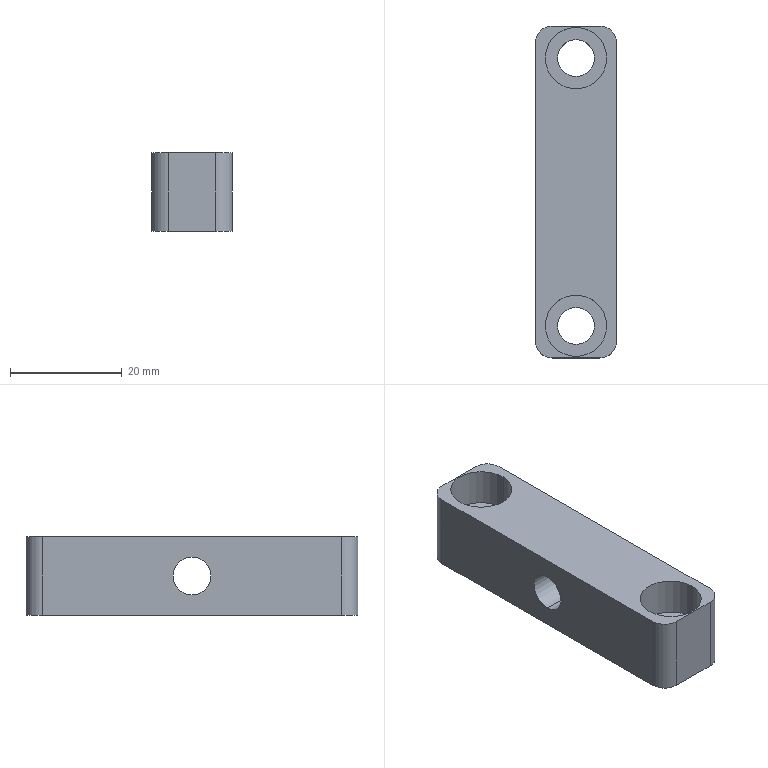Part | SolidWorks | features HoleWzd 2, Extrusion 1, Fillet 1 | 1 solid | 22 faces | box 14.5 x 59.5 x 14 mm | volume 9659 mm3 | cylinder 14 | plane 8 | commonest cylinder face diameters 6 x4 6.6 x4 11 x4 6.8 x2
STEP:
#1=CARTESIAN_POINT('',(7.25,0.,3.6));
#2=VERTEX_POINT('',#1);
#3=CARTESIAN_POINT('',(7.25,0.,10.4));
#4=VERTEX_POINT('',#3);
#5=CARTESIAN_POINT('',(7.25,0.,7.));
#6=DIRECTION('',(-1.,0.,0.));
#7=DIRECTION('',(0.,0.,1.));
#8=AXIS2_PLACEMENT_3D('',#5,#6,#7);
#9=CIRCLE('',#8,3.4);
#10=EDGE_CURVE('',#2,#4,#9,.T.);
#11=ORIENTED_EDGE('',*,*,#10,.F.);
#12=CARTESIAN_POINT('',(-7.25,0.,3.6));
#13=VERTEX_POINT('',#12);
#14=CARTESIAN_POINT('',(-7.25,0.,3.6));
#15=DIRECTION('',(-1.,0.,0.));
#16=VECTOR('',#15,1000.);
#17=LINE('',#14,#16);
#18=EDGE_CURVE('',#2,#13,#17,.T.);
#19=ORIENTED_EDGE('',*,*,#18,.T.);
#20=CARTESIAN_POINT('',(-7.25,0.,10.4));
#21=VERTEX_POINT('',#20);
#22=CARTESIAN_POINT('',(-7.25,0.,7.));
#23=DIRECTION('',(-1.,0.,0.));
#24=DIRECTION('',(0.,0.,1.));
#25=AXIS2_PLACEMENT_3D('',#22,#23,#24);
#26=CIRCLE('',#25,3.4);
#27=EDGE_CURVE('',#13,#21,#26,.T.);
#28=ORIENTED_EDGE('',*,*,#27,.T.);
#29=CARTESIAN_POINT('',(-7.25,0.,10.4));
#30=DIRECTION('',(-1.,0.,0.));
#31=VECTOR('',#30,1000.);
#32=LINE('',#29,#31);
#33=EDGE_CURVE('',#4,#21,#32,.T.);
#34=ORIENTED_EDGE('',*,*,#33,.F.);
#35=EDGE_LOOP('',(#11,#19,#28,#34));
#36=FACE_OUTER_BOUND('',#35,.T.);
#37=CARTESIAN_POINT('',(-7.25,0.,7.));
#38=DIRECTION('',(-1.,0.,0.));
#39=DIRECTION('',(0.,0.,1.));
#40=AXIS2_PLACEMENT_3D('',#37,#38,#39);
#41=CYLINDRICAL_SURFACE('',#40,3.4);
#42=ADVANCED_FACE('',(#36),#41,.F.);
#43=CARTESIAN_POINT('',(-5.5,24.,7.2));
#44=VERTEX_POINT('',#43);
#45=CARTESIAN_POINT('',(5.5,24.,7.2));
#46=VERTEX_POINT('',#45);
#47=CARTESIAN_POINT('',(0.,24.,7.2));
#48=DIRECTION('',(0.,0.,1.));
#49=DIRECTION('',(1.,0.,0.));
#50=AXIS2_PLACEMENT_3D('',#47,#48,#49);
#51=CIRCLE('',#50,5.5);
#52=EDGE_CURVE('',#44,#46,#51,.T.);
#53=ORIENTED_EDGE('',*,*,#52,.F.);
#54=CARTESIAN_POINT('',(-5.5,24.,14.));
#55=VERTEX_POINT('',#54);
#56=CARTESIAN_POINT('',(-5.5,24.,14.));
#57=DIRECTION('',(0.,0.,1.));
#58=VECTOR('',#57,1000.);
#59=LINE('',#56,#58);
#60=EDGE_CURVE('',#44,#55,#59,.T.);
#61=ORIENTED_EDGE('',*,*,#60,.T.);
#62=CARTESIAN_POINT('',(5.5,24.,14.));
#63=VERTEX_POINT('',#62);
#64=CARTESIAN_POINT('',(0.,24.,14.));
#65=DIRECTION('',(0.,0.,1.));
#66=DIRECTION('',(1.,0.,0.));
#67=AXIS2_PLACEMENT_3D('',#64,#65,#66);
#68=CIRCLE('',#67,5.5);
#69=EDGE_CURVE('',#55,#63,#68,.T.);
#70=ORIENTED_EDGE('',*,*,#69,.T.);
#71=CARTESIAN_POINT('',(5.5,24.,14.));
#72=DIRECTION('',(0.,0.,1.));
#73=VECTOR('',#72,1000.);
#74=LINE('',#71,#73);
#75=EDGE_CURVE('',#46,#63,#74,.T.);
#76=ORIENTED_EDGE('',*,*,#75,.F.);
#77=EDGE_LOOP('',(#53,#61,#70,#76));
#78=FACE_OUTER_BOUND('',#77,.T.);
#79=CARTESIAN_POINT('',(0.,24.,14.));
#80=DIRECTION('',(0.,0.,1.));
#81=DIRECTION('',(1.,0.,0.));
#82=AXIS2_PLACEMENT_3D('',#79,#80,#81);
#83=CYLINDRICAL_SURFACE('',#82,5.5);
#84=ADVANCED_FACE('',(#78),#83,.F.);
#85=CARTESIAN_POINT('',(-3.3,24.,0.));
#86=VERTEX_POINT('',#85);
#87=CARTESIAN_POINT('',(3.3,24.,0.));
#88=VERTEX_POINT('',#87);
#89=CARTESIAN_POINT('',(0.,24.,0.));
#90=DIRECTION('',(0.,0.,1.));
#91=DIRECTION('',(1.,0.,0.));
#92=AXIS2_PLACEMENT_3D('',#89,#90,#91);
#93=CIRCLE('',#92,3.3);
#94=EDGE_CURVE('',#86,#88,#93,.T.);
#95=ORIENTED_EDGE('',*,*,#94,.F.);
#96=CARTESIAN_POINT('',(-3.3,24.,7.2));
#97=VERTEX_POINT('',#96);
#98=CARTESIAN_POINT('',(-3.3,24.,14.));
#99=DIRECTION('',(0.,0.,1.));
#100=VECTOR('',#99,1000.);
#101=LINE('',#98,#100);
#102=EDGE_CURVE('',#86,#97,#101,.T.);
#103=ORIENTED_EDGE('',*,*,#102,.T.);
#104=CARTESIAN_POINT('',(3.3,24.,7.2));
#105=VERTEX_POINT('',#104);
#106=CARTESIAN_POINT('',(0.,24.,7.2));
#107=DIRECTION('',(0.,0.,1.));
#108=DIRECTION('',(1.,0.,0.));
#109=AXIS2_PLACEMENT_3D('',#106,#107,#108);
#110=CIRCLE('',#109,3.3);
#111=EDGE_CURVE('',#97,#105,#110,.T.);
#112=ORIENTED_EDGE('',*,*,#111,.T.);
#113=CARTESIAN_POINT('',(3.3,24.,14.));
#114=DIRECTION('',(0.,0.,1.));
#115=VECTOR('',#114,1000.);
#116=LINE('',#113,#115);
#117=EDGE_CURVE('',#88,#105,#116,.T.);
#118=ORIENTED_EDGE('',*,*,#117,.F.);
#119=EDGE_LOOP('',(#95,#103,#112,#118));
#120=FACE_OUTER_BOUND('',#119,.T.);
#121=CARTESIAN_POINT('',(0.,24.,14.));
#122=DIRECTION('',(0.,0.,1.));
#123=DIRECTION('',(1.,0.,0.));
#124=AXIS2_PLACEMENT_3D('',#121,#122,#123);
#125=CYLINDRICAL_SURFACE('',#124,3.3);
#126=ADVANCED_FACE('',(#120),#125,.F.);
#127=CARTESIAN_POINT('',(-5.5,-24.,7.2));
#128=VERTEX_POINT('',#127);
#129=CARTESIAN_POINT('',(5.5,-24.,7.2));
#130=VERTEX_POINT('',#129);
#131=CARTESIAN_POINT('',(0.,-24.,7.2));
#132=DIRECTION('',(0.,0.,1.));
#133=DIRECTION('',(1.,0.,0.));
#134=AXIS2_PLACEMENT_3D('',#131,#132,#133);
#135=CIRCLE('',#134,5.5);
#136=EDGE_CURVE('',#128,#130,#135,.T.);
#137=ORIENTED_EDGE('',*,*,#136,.F.);
#138=CARTESIAN_POINT('',(-5.5,-24.,14.));
#139=VERTEX_POINT('',#138);
#140=CARTESIAN_POINT('',(-5.5,-24.,14.));
#141=DIRECTION('',(0.,0.,1.));
#142=VECTOR('',#141,1000.);
#143=LINE('',#140,#142);
#144=EDGE_CURVE('',#128,#139,#143,.T.);
#145=ORIENTED_EDGE('',*,*,#144,.T.);
#146=CARTESIAN_POINT('',(5.5,-24.,14.));
#147=VERTEX_POINT('',#146);
#148=CARTESIAN_POINT('',(0.,-24.,14.));
#149=DIRECTION('',(0.,0.,1.));
#150=DIRECTION('',(1.,0.,0.));
#151=AXIS2_PLACEMENT_3D('',#148,#149,#150);
#152=CIRCLE('',#151,5.5);
#153=EDGE_CURVE('',#139,#147,#152,.T.);
#154=ORIENTED_EDGE('',*,*,#153,.T.);
#155=CARTESIAN_POINT('',(5.5,-24.,14.));
#156=DIRECTION('',(0.,0.,1.));
#157=VECTOR('',#156,1000.);
#158=LINE('',#155,#157);
#159=EDGE_CURVE('',#130,#147,#158,.T.);
#160=ORIENTED_EDGE('',*,*,#159,.F.);
#161=EDGE_LOOP('',(#137,#145,#154,#160));
#162=FACE_OUTER_BOUND('',#161,.T.);
#163=CARTESIAN_POINT('',(0.,-24.,14.));
#164=DIRECTION('',(0.,0.,1.));
#165=DIRECTION('',(1.,0.,0.));
#166=AXIS2_PLACEMENT_3D('',#163,#164,#165);
#167=CYLINDRICAL_SURFACE('',#166,5.5);
#168=ADVANCED_FACE('',(#162),#167,.F.);
#169=CARTESIAN_POINT('',(-3.3,-24.,0.));
#170=VERTEX_POINT('',#169);
#171=CARTESIAN_POINT('',(3.3,-24.,0.));
#172=VERTEX_POINT('',#171);
#173=CARTESIAN_POINT('',(0.,-24.,0.));
#174=DIRECTION('',(0.,0.,1.));
#175=DIRECTION('',(1.,0.,0.));
#176=AXIS2_PLACEMENT_3D('',#173,#174,#175);
#177=CIRCLE('',#176,3.3);
#178=EDGE_CURVE('',#170,#172,#177,.T.);
#179=ORIENTED_EDGE('',*,*,#178,.F.);
#180=CARTESIAN_POINT('',(-3.3,-24.,7.2));
#181=VERTEX_POINT('',#180);
#182=CARTESIAN_POINT('',(-3.3,-24.,14.));
#183=DIRECTION('',(0.,0.,1.));
#184=VECTOR('',#183,1000.);
#185=LINE('',#182,#184);
#186=EDGE_CURVE('',#170,#181,#185,.T.);
#187=ORIENTED_EDGE('',*,*,#186,.T.);
#188=CARTESIAN_POINT('',(3.3,-24.,7.2));
#189=VERTEX_POINT('',#188);
#190=CARTESIAN_POINT('',(0.,-24.,7.2));
#191=DIRECTION('',(0.,0.,1.));
#192=DIRECTION('',(1.,0.,0.));
#193=AXIS2_PLACEMENT_3D('',#190,#191,#192);
#194=CIRCLE('',#193,3.3);
#195=EDGE_CURVE('',#181,#189,#194,.T.);
#196=ORIENTED_EDGE('',*,*,#195,.T.);
#197=CARTESIAN_POINT('',(3.3,-24.,14.));
#198=DIRECTION('',(0.,0.,1.));
#199=VECTOR('',#198,1000.);
#200=LINE('',#197,#199);
#201=EDGE_CURVE('',#172,#189,#200,.T.);
#202=ORIENTED_EDGE('',*,*,#201,.F.);
#203=EDGE_LOOP('',(#179,#187,#196,#202));
#204=FACE_OUTER_BOUND('',#203,.T.);
#205=CARTESIAN_POINT('',(0.,-24.,14.));
#206=DIRECTION('',(0.,0.,1.));
#207=DIRECTION('',(1.,0.,0.));
#208=AXIS2_PLACEMENT_3D('',#205,#206,#207);
#209=CYLINDRICAL_SURFACE('',#208,3.3);
#210=ADVANCED_FACE('',(#204),#209,.F.);
#211=CARTESIAN_POINT('',(7.25,0.,7.));
#212=DIRECTION('',(-1.,0.,0.));
#213=DIRECTION('',(0.,0.,1.));
#214=AXIS2_PLACEMENT_3D('',#211,#212,#213);
#215=CIRCLE('',#214,3.4);
#216=EDGE_CURVE('',#4,#2,#215,.T.);
#217=ORIENTED_EDGE('',*,*,#216,.T.);
#218=ORIENTED_EDGE('',*,*,#10,.T.);
#219=EDGE_LOOP('',(#217,#218));
#220=FACE_BOUND('',#219,.T.);
#221=CARTESIAN_POINT('',(7.25,-26.75,14.));
#222=VERTEX_POINT('',#221);
#223=CARTESIAN_POINT('',(7.25,26.75,14.));
#224=VERTEX_POINT('',#223);
#225=CARTESIAN_POINT('',(7.25,29.75,14.));
#226=DIRECTION('',(0.,1.,0.));
#227=VECTOR('',#226,1000.);
#228=LINE('',#225,#227);
#229=EDGE_CURVE('',#222,#224,#228,.T.);
#230=ORIENTED_EDGE('',*,*,#229,.F.);
#231=CARTESIAN_POINT('',(7.25,-26.75,0.));
#232=VERTEX_POINT('',#231);
#233=CARTESIAN_POINT('',(7.25,-26.75,14.));
#234=DIRECTION('',(0.,0.,-1.));
#235=VECTOR('',#234,1000.);
#236=LINE('',#233,#235);
#237=EDGE_CURVE('',#222,#232,#236,.T.);
#238=ORIENTED_EDGE('',*,*,#237,.T.);
#239=CARTESIAN_POINT('',(7.25,26.75,0.));
#240=VERTEX_POINT('',#239);
#241=CARTESIAN_POINT('',(7.25,29.75,0.));
#242=DIRECTION('',(0.,1.,0.));
#243=VECTOR('',#242,1000.);
#244=LINE('',#241,#243);
#245=EDGE_CURVE('',#232,#240,#244,.T.);
#246=ORIENTED_EDGE('',*,*,#245,.T.);
#247=CARTESIAN_POINT('',(7.25,26.75,14.));
#248=DIRECTION('',(0.,0.,1.));
#249=VECTOR('',#248,1000.);
#250=LINE('',#247,#249);
#251=EDGE_CURVE('',#240,#224,#250,.T.);
#252=ORIENTED_EDGE('',*,*,#251,.T.);
#253=EDGE_LOOP('',(#230,#238,#246,#252));
#254=FACE_OUTER_BOUND('',#253,.T.);
#255=CARTESIAN_POINT('',(7.25,29.75,14.));
#256=DIRECTION('',(-1.,0.,0.));
#257=DIRECTION('',(0.,-1.,0.));
#258=AXIS2_PLACEMENT_3D('',#255,#256,#257);
#259=PLANE('',#258);
#260=ADVANCED_FACE('',(#220,#254),#259,.F.);
#261=CARTESIAN_POINT('',(4.25,29.75,14.));
#262=VERTEX_POINT('',#261);
#263=CARTESIAN_POINT('',(-4.25,29.75,14.));
#264=VERTEX_POINT('',#263);
#265=CARTESIAN_POINT('',(-7.25,29.75,14.));
#266=DIRECTION('',(-1.,0.,0.));
#267=VECTOR('',#266,1000.);
#268=LINE('',#265,#267);
#269=EDGE_CURVE('',#262,#264,#268,.T.);
#270=ORIENTED_EDGE('',*,*,#269,.F.);
#271=CARTESIAN_POINT('',(4.25,29.75,0.));
#272=VERTEX_POINT('',#271);
#273=CARTESIAN_POINT('',(4.25,29.75,14.));
#274=DIRECTION('',(0.,0.,-1.));
#275=VECTOR('',#274,1000.);
#276=LINE('',#273,#275);
#277=EDGE_CURVE('',#262,#272,#276,.T.);
#278=ORIENTED_EDGE('',*,*,#277,.T.);
#279=CARTESIAN_POINT('',(-4.25,29.75,0.));
#280=VERTEX_POINT('',#279);
#281=CARTESIAN_POINT('',(-7.25,29.75,0.));
#282=DIRECTION('',(-1.,0.,0.));
#283=VECTOR('',#282,1000.);
#284=LINE('',#281,#283);
#285=EDGE_CURVE('',#272,#280,#284,.T.);
#286=ORIENTED_EDGE('',*,*,#285,.T.);
#287=CARTESIAN_POINT('',(-4.25,29.75,14.));
#288=DIRECTION('',(0.,0.,1.));
#289=VECTOR('',#288,1000.);
#290=LINE('',#287,#289);
#291=EDGE_CURVE('',#280,#264,#290,.T.);
#292=ORIENTED_EDGE('',*,*,#291,.T.);
#293=EDGE_LOOP('',(#270,#278,#286,#292));
#294=FACE_OUTER_BOUND('',#293,.T.);
#295=CARTESIAN_POINT('',(-7.25,29.75,14.));
#296=DIRECTION('',(0.,-1.,0.));
#297=DIRECTION('',(0.,0.,-1.));
#298=AXIS2_PLACEMENT_3D('',#295,#296,#297);
#299=PLANE('',#298);
#300=ADVANCED_FACE('',(#294),#299,.F.);
#301=CARTESIAN_POINT('',(-7.25,0.,7.));
#302=DIRECTION('',(-1.,0.,0.));
#303=DIRECTION('',(0.,0.,1.));
#304=AXIS2_PLACEMENT_3D('',#301,#302,#303);
#305=CIRCLE('',#304,3.4);
#306=EDGE_CURVE('',#21,#13,#305,.T.);
#307=ORIENTED_EDGE('',*,*,#306,.F.);
#308=ORIENTED_EDGE('',*,*,#27,.F.);
#309=EDGE_LOOP('',(#307,#308));
#310=FACE_BOUND('',#309,.T.);
#311=CARTESIAN_POINT('',(-7.25,26.75,0.));
#312=VERTEX_POINT('',#311);
#313=CARTESIAN_POINT('',(-7.25,-26.75,0.));
#314=VERTEX_POINT('',#313);
#315=CARTESIAN_POINT('',(-7.25,29.75,0.));
#316=DIRECTION('',(0.,-1.,0.));
#317=VECTOR('',#316,1000.);
#318=LINE('',#315,#317);
#319=EDGE_CURVE('',#312,#314,#318,.T.);
#320=ORIENTED_EDGE('',*,*,#319,.T.);
#321=CARTESIAN_POINT('',(-7.25,-26.75,14.));
#322=VERTEX_POINT('',#321);
#323=CARTESIAN_POINT('',(-7.25,-26.75,14.));
#324=DIRECTION('',(0.,0.,1.));
#325=VECTOR('',#324,1000.);
#326=LINE('',#323,#325);
#327=EDGE_CURVE('',#314,#322,#326,.T.);
#328=ORIENTED_EDGE('',*,*,#327,.T.);
#329=CARTESIAN_POINT('',(-7.25,26.75,14.));
#330=VERTEX_POINT('',#329);
#331=CARTESIAN_POINT('',(-7.25,29.75,14.));
#332=DIRECTION('',(0.,-1.,0.));
#333=VECTOR('',#332,1000.);
#334=LINE('',#331,#333);
#335=EDGE_CURVE('',#330,#322,#334,.T.);
#336=ORIENTED_EDGE('',*,*,#335,.F.);
#337=CARTESIAN_POINT('',(-7.25,26.75,14.));
#338=DIRECTION('',(0.,0.,-1.));
#339=VECTOR('',#338,1000.);
#340=LINE('',#337,#339);
#341=EDGE_CURVE('',#330,#312,#340,.T.);
#342=ORIENTED_EDGE('',*,*,#341,.T.);
#343=EDGE_LOOP('',(#320,#328,#336,#342));
#344=FACE_OUTER_BOUND('',#343,.T.);
#345=CARTESIAN_POINT('',(-7.25,29.75,14.));
#346=DIRECTION('',(1.,0.,0.));
#347=DIRECTION('',(0.,1.,0.));
#348=AXIS2_PLACEMENT_3D('',#345,#346,#347);
#349=PLANE('',#348);
#350=ADVANCED_FACE('',(#310,#344),#349,.F.);
#351=CARTESIAN_POINT('',(-4.25,-29.75,0.));
#352=VERTEX_POINT('',#351);
#353=CARTESIAN_POINT('',(4.25,-29.75,0.));
#354=VERTEX_POINT('',#353);
#355=CARTESIAN_POINT('',(-7.25,-29.75,0.));
#356=DIRECTION('',(1.,0.,0.));
#357=VECTOR('',#356,1000.);
#358=LINE('',#355,#357);
#359=EDGE_CURVE('',#352,#354,#358,.T.);
#360=ORIENTED_EDGE('',*,*,#359,.T.);
#361=CARTESIAN_POINT('',(4.25,-29.75,14.));
#362=VERTEX_POINT('',#361);
#363=CARTESIAN_POINT('',(4.25,-29.75,14.));
#364=DIRECTION('',(0.,0.,1.));
#365=VECTOR('',#364,1000.);
#366=LINE('',#363,#365);
#367=EDGE_CURVE('',#354,#362,#366,.T.);
#368=ORIENTED_EDGE('',*,*,#367,.T.);
#369=CARTESIAN_POINT('',(-4.25,-29.75,14.));
#370=VERTEX_POINT('',#369);
#371=CARTESIAN_POINT('',(-7.25,-29.75,14.));
#372=DIRECTION('',(1.,0.,0.));
#373=VECTOR('',#372,1000.);
#374=LINE('',#371,#373);
#375=EDGE_CURVE('',#370,#362,#374,.T.);
#376=ORIENTED_EDGE('',*,*,#375,.F.);
#377=CARTESIAN_POINT('',(-4.25,-29.75,14.));
#378=DIRECTION('',(0.,0.,-1.));
#379=VECTOR('',#378,1000.);
#380=LINE('',#377,#379);
#381=EDGE_CURVE('',#370,#352,#380,.T.);
#382=ORIENTED_EDGE('',*,*,#381,.T.);
#383=EDGE_LOOP('',(#360,#368,#376,#382));
#384=FACE_OUTER_BOUND('',#383,.T.);
#385=CARTESIAN_POINT('',(-7.25,-29.75,14.));
#386=DIRECTION('',(0.,1.,0.));
#387=DIRECTION('',(0.,0.,1.));
#388=AXIS2_PLACEMENT_3D('',#385,#386,#387);
#389=PLANE('',#388);
#390=ADVANCED_FACE('',(#384),#389,.F.);
#391=CARTESIAN_POINT('',(0.,24.,14.));
#392=DIRECTION('',(0.,0.,1.));
#393=DIRECTION('',(1.,0.,0.));
#394=AXIS2_PLACEMENT_3D('',#391,#392,#393);
#395=CIRCLE('',#394,5.5);
#396=EDGE_CURVE('',#63,#55,#395,.T.);
#397=ORIENTED_EDGE('',*,*,#396,.F.);
#398=ORIENTED_EDGE('',*,*,#69,.F.);
#399=EDGE_LOOP('',(#397,#398));
#400=FACE_BOUND('',#399,.T.);
#401=CARTESIAN_POINT('',(0.,-24.,14.));
#402=DIRECTION('',(0.,0.,1.));
#403=DIRECTION('',(1.,0.,0.));
#404=AXIS2_PLACEMENT_3D('',#401,#402,#403);
#405=CIRCLE('',#404,5.5);
#406=EDGE_CURVE('',#147,#139,#405,.T.);
#407=ORIENTED_EDGE('',*,*,#406,.F.);
#408=ORIENTED_EDGE('',*,*,#153,.F.);
#409=EDGE_LOOP('',(#407,#408));
#410=FACE_BOUND('',#409,.T.);
#411=ORIENTED_EDGE('',*,*,#375,.T.);
#412=CARTESIAN_POINT('',(4.25,-26.75,14.));
#413=DIRECTION('',(0.,0.,1.));
#414=DIRECTION('',(1.,0.,0.));
#415=AXIS2_PLACEMENT_3D('',#412,#413,#414);
#416=CIRCLE('',#415,3.);
#417=EDGE_CURVE('',#362,#222,#416,.T.);
#418=ORIENTED_EDGE('',*,*,#417,.T.);
#419=ORIENTED_EDGE('',*,*,#229,.T.);
#420=CARTESIAN_POINT('',(4.25,26.75,14.));
#421=DIRECTION('',(0.,0.,1.));
#422=DIRECTION('',(1.,0.,0.));
#423=AXIS2_PLACEMENT_3D('',#420,#421,#422);
#424=CIRCLE('',#423,3.);
#425=EDGE_CURVE('',#224,#262,#424,.T.);
#426=ORIENTED_EDGE('',*,*,#425,.T.);
#427=ORIENTED_EDGE('',*,*,#269,.T.);
#428=CARTESIAN_POINT('',(-4.25,26.75,14.));
#429=DIRECTION('',(0.,0.,1.));
#430=DIRECTION('',(1.,0.,0.));
#431=AXIS2_PLACEMENT_3D('',#428,#429,#430);
#432=CIRCLE('',#431,3.);
#433=EDGE_CURVE('',#264,#330,#432,.T.);
#434=ORIENTED_EDGE('',*,*,#433,.T.);
#435=ORIENTED_EDGE('',*,*,#335,.T.);
#436=CARTESIAN_POINT('',(-4.25,-26.75,14.));
#437=DIRECTION('',(0.,0.,1.));
#438=DIRECTION('',(1.,0.,0.));
#439=AXIS2_PLACEMENT_3D('',#436,#437,#438);
#440=CIRCLE('',#439,3.);
#441=EDGE_CURVE('',#322,#370,#440,.T.);
#442=ORIENTED_EDGE('',*,*,#441,.T.);
#443=EDGE_LOOP('',(#411,#418,#419,#426,#427,#434,#435,#442));
#444=FACE_OUTER_BOUND('',#443,.T.);
#445=CARTESIAN_POINT('',(0.,0.,14.));
#446=DIRECTION('',(0.,0.,1.));
#447=DIRECTION('',(1.,0.,0.));
#448=AXIS2_PLACEMENT_3D('',#445,#446,#447);
#449=PLANE('',#448);
#450=ADVANCED_FACE('',(#400,#410,#444),#449,.T.);
#451=CARTESIAN_POINT('',(0.,24.,0.));
#452=DIRECTION('',(0.,0.,1.));
#453=DIRECTION('',(1.,0.,0.));
#454=AXIS2_PLACEMENT_3D('',#451,#452,#453);
#455=CIRCLE('',#454,3.3);
#456=EDGE_CURVE('',#88,#86,#455,.T.);
#457=ORIENTED_EDGE('',*,*,#456,.T.);
#458=ORIENTED_EDGE('',*,*,#94,.T.);
#459=EDGE_LOOP('',(#457,#458));
#460=FACE_BOUND('',#459,.T.);
#461=CARTESIAN_POINT('',(0.,-24.,0.));
#462=DIRECTION('',(0.,0.,1.));
#463=DIRECTION('',(1.,0.,0.));
#464=AXIS2_PLACEMENT_3D('',#461,#462,#463);
#465=CIRCLE('',#464,3.3);
#466=EDGE_CURVE('',#172,#170,#465,.T.);
#467=ORIENTED_EDGE('',*,*,#466,.T.);
#468=ORIENTED_EDGE('',*,*,#178,.T.);
#469=EDGE_LOOP('',(#467,#468));
#470=FACE_BOUND('',#469,.T.);
#471=ORIENTED_EDGE('',*,*,#245,.F.);
#472=CARTESIAN_POINT('',(4.25,-26.75,0.));
#473=DIRECTION('',(0.,0.,-1.));
#474=DIRECTION('',(1.,0.,0.));
#475=AXIS2_PLACEMENT_3D('',#472,#473,#474);
#476=CIRCLE('',#475,3.);
#477=EDGE_CURVE('',#232,#354,#476,.T.);
#478=ORIENTED_EDGE('',*,*,#477,.T.);
#479=ORIENTED_EDGE('',*,*,#359,.F.);
#480=CARTESIAN_POINT('',(-4.25,-26.75,0.));
#481=DIRECTION('',(0.,0.,-1.));
#482=DIRECTION('',(1.,0.,0.));
#483=AXIS2_PLACEMENT_3D('',#480,#481,#482);
#484=CIRCLE('',#483,3.);
#485=EDGE_CURVE('',#352,#314,#484,.T.);
#486=ORIENTED_EDGE('',*,*,#485,.T.);
#487=ORIENTED_EDGE('',*,*,#319,.F.);
#488=CARTESIAN_POINT('',(-4.25,26.75,0.));
#489=DIRECTION('',(0.,0.,-1.));
#490=DIRECTION('',(1.,0.,0.));
#491=AXIS2_PLACEMENT_3D('',#488,#489,#490);
#492=CIRCLE('',#491,3.);
#493=EDGE_CURVE('',#312,#280,#492,.T.);
#494=ORIENTED_EDGE('',*,*,#493,.T.);
#495=ORIENTED_EDGE('',*,*,#285,.F.);
#496=CARTESIAN_POINT('',(4.25,26.75,0.));
#497=DIRECTION('',(0.,0.,-1.));
#498=DIRECTION('',(1.,0.,0.));
#499=AXIS2_PLACEMENT_3D('',#496,#497,#498);
#500=CIRCLE('',#499,3.);
#501=EDGE_CURVE('',#272,#240,#500,.T.);
#502=ORIENTED_EDGE('',*,*,#501,.T.);
#503=EDGE_LOOP('',(#471,#478,#479,#486,#487,#494,#495,#502));
#504=FACE_OUTER_BOUND('',#503,.T.);
#505=CARTESIAN_POINT('',(0.,0.,0.));
#506=DIRECTION('',(0.,0.,1.));
#507=DIRECTION('',(1.,0.,0.));
#508=AXIS2_PLACEMENT_3D('',#505,#506,#507);
#509=PLANE('',#508);
#510=ADVANCED_FACE('',(#460,#470,#504),#509,.F.);
#511=ORIENTED_EDGE('',*,*,#417,.F.);
#512=ORIENTED_EDGE('',*,*,#367,.F.);
#513=ORIENTED_EDGE('',*,*,#477,.F.);
#514=ORIENTED_EDGE('',*,*,#237,.F.);
#515=EDGE_LOOP('',(#511,#512,#513,#514));
#516=FACE_OUTER_BOUND('',#515,.T.);
#517=CARTESIAN_POINT('',(4.25,-26.75,14.));
#518=DIRECTION('',(0.,0.,-1.));
#519=DIRECTION('',(-1.,0.,0.));
#520=AXIS2_PLACEMENT_3D('',#517,#518,#519);
#521=CYLINDRICAL_SURFACE('',#520,3.);
#522=ADVANCED_FACE('',(#516),#521,.T.);
#523=ORIENTED_EDGE('',*,*,#441,.F.);
#524=ORIENTED_EDGE('',*,*,#327,.F.);
#525=ORIENTED_EDGE('',*,*,#485,.F.);
#526=ORIENTED_EDGE('',*,*,#381,.F.);
#527=EDGE_LOOP('',(#523,#524,#525,#526));
#528=FACE_OUTER_BOUND('',#527,.T.);
#529=CARTESIAN_POINT('',(-4.25,-26.75,14.));
#530=DIRECTION('',(0.,0.,-1.));
#531=DIRECTION('',(-1.,0.,0.));
#532=AXIS2_PLACEMENT_3D('',#529,#530,#531);
#533=CYLINDRICAL_SURFACE('',#532,3.);
#534=ADVANCED_FACE('',(#528),#533,.T.);
#535=ORIENTED_EDGE('',*,*,#425,.F.);
#536=ORIENTED_EDGE('',*,*,#251,.F.);
#537=ORIENTED_EDGE('',*,*,#501,.F.);
#538=ORIENTED_EDGE('',*,*,#277,.F.);
#539=EDGE_LOOP('',(#535,#536,#537,#538));
#540=FACE_OUTER_BOUND('',#539,.T.);
#541=CARTESIAN_POINT('',(4.25,26.75,14.));
#542=DIRECTION('',(0.,0.,-1.));
#543=DIRECTION('',(-1.,0.,0.));
#544=AXIS2_PLACEMENT_3D('',#541,#542,#543);
#545=CYLINDRICAL_SURFACE('',#544,3.);
#546=ADVANCED_FACE('',(#540),#545,.T.);
#547=ORIENTED_EDGE('',*,*,#433,.F.);
#548=ORIENTED_EDGE('',*,*,#291,.F.);
#549=ORIENTED_EDGE('',*,*,#493,.F.);
#550=ORIENTED_EDGE('',*,*,#341,.F.);
#551=EDGE_LOOP('',(#547,#548,#549,#550));
#552=FACE_OUTER_BOUND('',#551,.T.);
#553=CARTESIAN_POINT('',(-4.25,26.75,14.));
#554=DIRECTION('',(0.,0.,-1.));
#555=DIRECTION('',(-1.,0.,0.));
#556=AXIS2_PLACEMENT_3D('',#553,#554,#555);
#557=CYLINDRICAL_SURFACE('',#556,3.);
#558=ADVANCED_FACE('',(#552),#557,.T.);
#559=ORIENTED_EDGE('',*,*,#186,.F.);
#560=ORIENTED_EDGE('',*,*,#466,.F.);
#561=ORIENTED_EDGE('',*,*,#201,.T.);
#562=CARTESIAN_POINT('',(0.,-24.,7.2));
#563=DIRECTION('',(0.,0.,1.));
#564=DIRECTION('',(1.,0.,0.));
#565=AXIS2_PLACEMENT_3D('',#562,#563,#564);
#566=CIRCLE('',#565,3.3);
#567=EDGE_CURVE('',#189,#181,#566,.T.);
#568=ORIENTED_EDGE('',*,*,#567,.T.);
#569=EDGE_LOOP('',(#559,#560,#561,#568));
#570=FACE_OUTER_BOUND('',#569,.T.);
#571=CARTESIAN_POINT('',(0.,-24.,14.));
#572=DIRECTION('',(0.,0.,1.));
#573=DIRECTION('',(1.,0.,0.));
#574=AXIS2_PLACEMENT_3D('',#571,#572,#573);
#575=CYLINDRICAL_SURFACE('',#574,3.3);
#576=ADVANCED_FACE('',(#570),#575,.F.);
#577=ORIENTED_EDGE('',*,*,#567,.F.);
#578=ORIENTED_EDGE('',*,*,#195,.F.);
#579=EDGE_LOOP('',(#577,#578));
#580=FACE_BOUND('',#579,.T.);
#581=CARTESIAN_POINT('',(0.,-24.,7.2));
#582=DIRECTION('',(0.,0.,1.));
#583=DIRECTION('',(1.,0.,0.));
#584=AXIS2_PLACEMENT_3D('',#581,#582,#583);
#585=CIRCLE('',#584,5.5);
#586=EDGE_CURVE('',#130,#128,#585,.T.);
#587=ORIENTED_EDGE('',*,*,#586,.T.);
#588=ORIENTED_EDGE('',*,*,#136,.T.);
#589=EDGE_LOOP('',(#587,#588));
#590=FACE_OUTER_BOUND('',#589,.T.);
#591=CARTESIAN_POINT('',(3.3,-24.,7.2));
#592=DIRECTION('',(0.,0.,-1.));
#593=DIRECTION('',(-1.,0.,0.));
#594=AXIS2_PLACEMENT_3D('',#591,#592,#593);
#595=PLANE('',#594);
#596=ADVANCED_FACE('',(#580,#590),#595,.F.);
#597=ORIENTED_EDGE('',*,*,#144,.F.);
#598=ORIENTED_EDGE('',*,*,#586,.F.);
#599=ORIENTED_EDGE('',*,*,#159,.T.);
#600=ORIENTED_EDGE('',*,*,#406,.T.);
#601=EDGE_LOOP('',(#597,#598,#599,#600));
#602=FACE_OUTER_BOUND('',#601,.T.);
#603=CARTESIAN_POINT('',(0.,-24.,14.));
#604=DIRECTION('',(0.,0.,1.));
#605=DIRECTION('',(1.,0.,0.));
#606=AXIS2_PLACEMENT_3D('',#603,#604,#605);
#607=CYLINDRICAL_SURFACE('',#606,5.5);
#608=ADVANCED_FACE('',(#602),#607,.F.);
#609=ORIENTED_EDGE('',*,*,#102,.F.);
#610=ORIENTED_EDGE('',*,*,#456,.F.);
#611=ORIENTED_EDGE('',*,*,#117,.T.);
#612=CARTESIAN_POINT('',(0.,24.,7.2));
#613=DIRECTION('',(0.,0.,1.));
#614=DIRECTION('',(1.,0.,0.));
#615=AXIS2_PLACEMENT_3D('',#612,#613,#614);
#616=CIRCLE('',#615,3.3);
#617=EDGE_CURVE('',#105,#97,#616,.T.);
#618=ORIENTED_EDGE('',*,*,#617,.T.);
#619=EDGE_LOOP('',(#609,#610,#611,#618));
#620=FACE_OUTER_BOUND('',#619,.T.);
#621=CARTESIAN_POINT('',(0.,24.,14.));
#622=DIRECTION('',(0.,0.,1.));
#623=DIRECTION('',(1.,0.,0.));
#624=AXIS2_PLACEMENT_3D('',#621,#622,#623);
#625=CYLINDRICAL_SURFACE('',#624,3.3);
#626=ADVANCED_FACE('',(#620),#625,.F.);
#627=ORIENTED_EDGE('',*,*,#617,.F.);
#628=ORIENTED_EDGE('',*,*,#111,.F.);
#629=EDGE_LOOP('',(#627,#628));
#630=FACE_BOUND('',#629,.T.);
#631=CARTESIAN_POINT('',(0.,24.,7.2));
#632=DIRECTION('',(0.,0.,1.));
#633=DIRECTION('',(1.,0.,0.));
#634=AXIS2_PLACEMENT_3D('',#631,#632,#633);
#635=CIRCLE('',#634,5.5);
#636=EDGE_CURVE('',#46,#44,#635,.T.);
#637=ORIENTED_EDGE('',*,*,#636,.T.);
#638=ORIENTED_EDGE('',*,*,#52,.T.);
#639=EDGE_LOOP('',(#637,#638));
#640=FACE_OUTER_BOUND('',#639,.T.);
#641=CARTESIAN_POINT('',(3.3,24.,7.2));
#642=DIRECTION('',(0.,0.,-1.));
#643=DIRECTION('',(-1.,0.,0.));
#644=AXIS2_PLACEMENT_3D('',#641,#642,#643);
#645=PLANE('',#644);
#646=ADVANCED_FACE('',(#630,#640),#645,.F.);
#647=ORIENTED_EDGE('',*,*,#60,.F.);
#648=ORIENTED_EDGE('',*,*,#636,.F.);
#649=ORIENTED_EDGE('',*,*,#75,.T.);
#650=ORIENTED_EDGE('',*,*,#396,.T.);
#651=EDGE_LOOP('',(#647,#648,#649,#650));
#652=FACE_OUTER_BOUND('',#651,.T.);
#653=CARTESIAN_POINT('',(0.,24.,14.));
#654=DIRECTION('',(0.,0.,1.));
#655=DIRECTION('',(1.,0.,0.));
#656=AXIS2_PLACEMENT_3D('',#653,#654,#655);
#657=CYLINDRICAL_SURFACE('',#656,5.5);
#658=ADVANCED_FACE('',(#652),#657,.F.);
#659=ORIENTED_EDGE('',*,*,#18,.F.);
#660=ORIENTED_EDGE('',*,*,#216,.F.);
#661=ORIENTED_EDGE('',*,*,#33,.T.);
#662=ORIENTED_EDGE('',*,*,#306,.T.);
#663=EDGE_LOOP('',(#659,#660,#661,#662));
#664=FACE_OUTER_BOUND('',#663,.T.);
#665=CARTESIAN_POINT('',(-7.25,0.,7.));
#666=DIRECTION('',(-1.,0.,0.));
#667=DIRECTION('',(0.,0.,1.));
#668=AXIS2_PLACEMENT_3D('',#665,#666,#667);
#669=CYLINDRICAL_SURFACE('',#668,3.4);
#670=ADVANCED_FACE('',(#664),#669,.F.);
#671=CLOSED_SHELL('',(#42,#84,#126,#168,#210,#260,#300,#350,#390,#450,#510,#522,#534,#546,#558,#576,#596,#608,#626,#646,#658,#670));
#672=MANIFOLD_SOLID_BREP('',#671);
#673=CARTESIAN_POINT('',(0.,0.,0.));
#674=DIRECTION('',(0.,0.,1.));
#675=DIRECTION('',(1.,0.,0.));
#676=AXIS2_PLACEMENT_3D('',#673,#674,#675);
#677=(LENGTH_UNIT()NAMED_UNIT(*)SI_UNIT(.MILLI.,.METRE.));
#678=UNCERTAINTY_MEASURE_WITH_UNIT(LENGTH_MEASURE(0.00001),#677,'','');
#679=(NAMED_UNIT(*)PLANE_ANGLE_UNIT()SI_UNIT($,.RADIAN.));
#680=(NAMED_UNIT(*)SI_UNIT($,.STERADIAN.)SOLID_ANGLE_UNIT());
#681=(GEOMETRIC_REPRESENTATION_CONTEXT(3)GLOBAL_UNCERTAINTY_ASSIGNED_CONTEXT((#678))GLOBAL_UNIT_ASSIGNED_CONTEXT((#677,#679,#680))REPRESENTATION_CONTEXT('',''));
#682=ADVANCED_BREP_SHAPE_REPRESENTATION('',(#672,#676),#681);